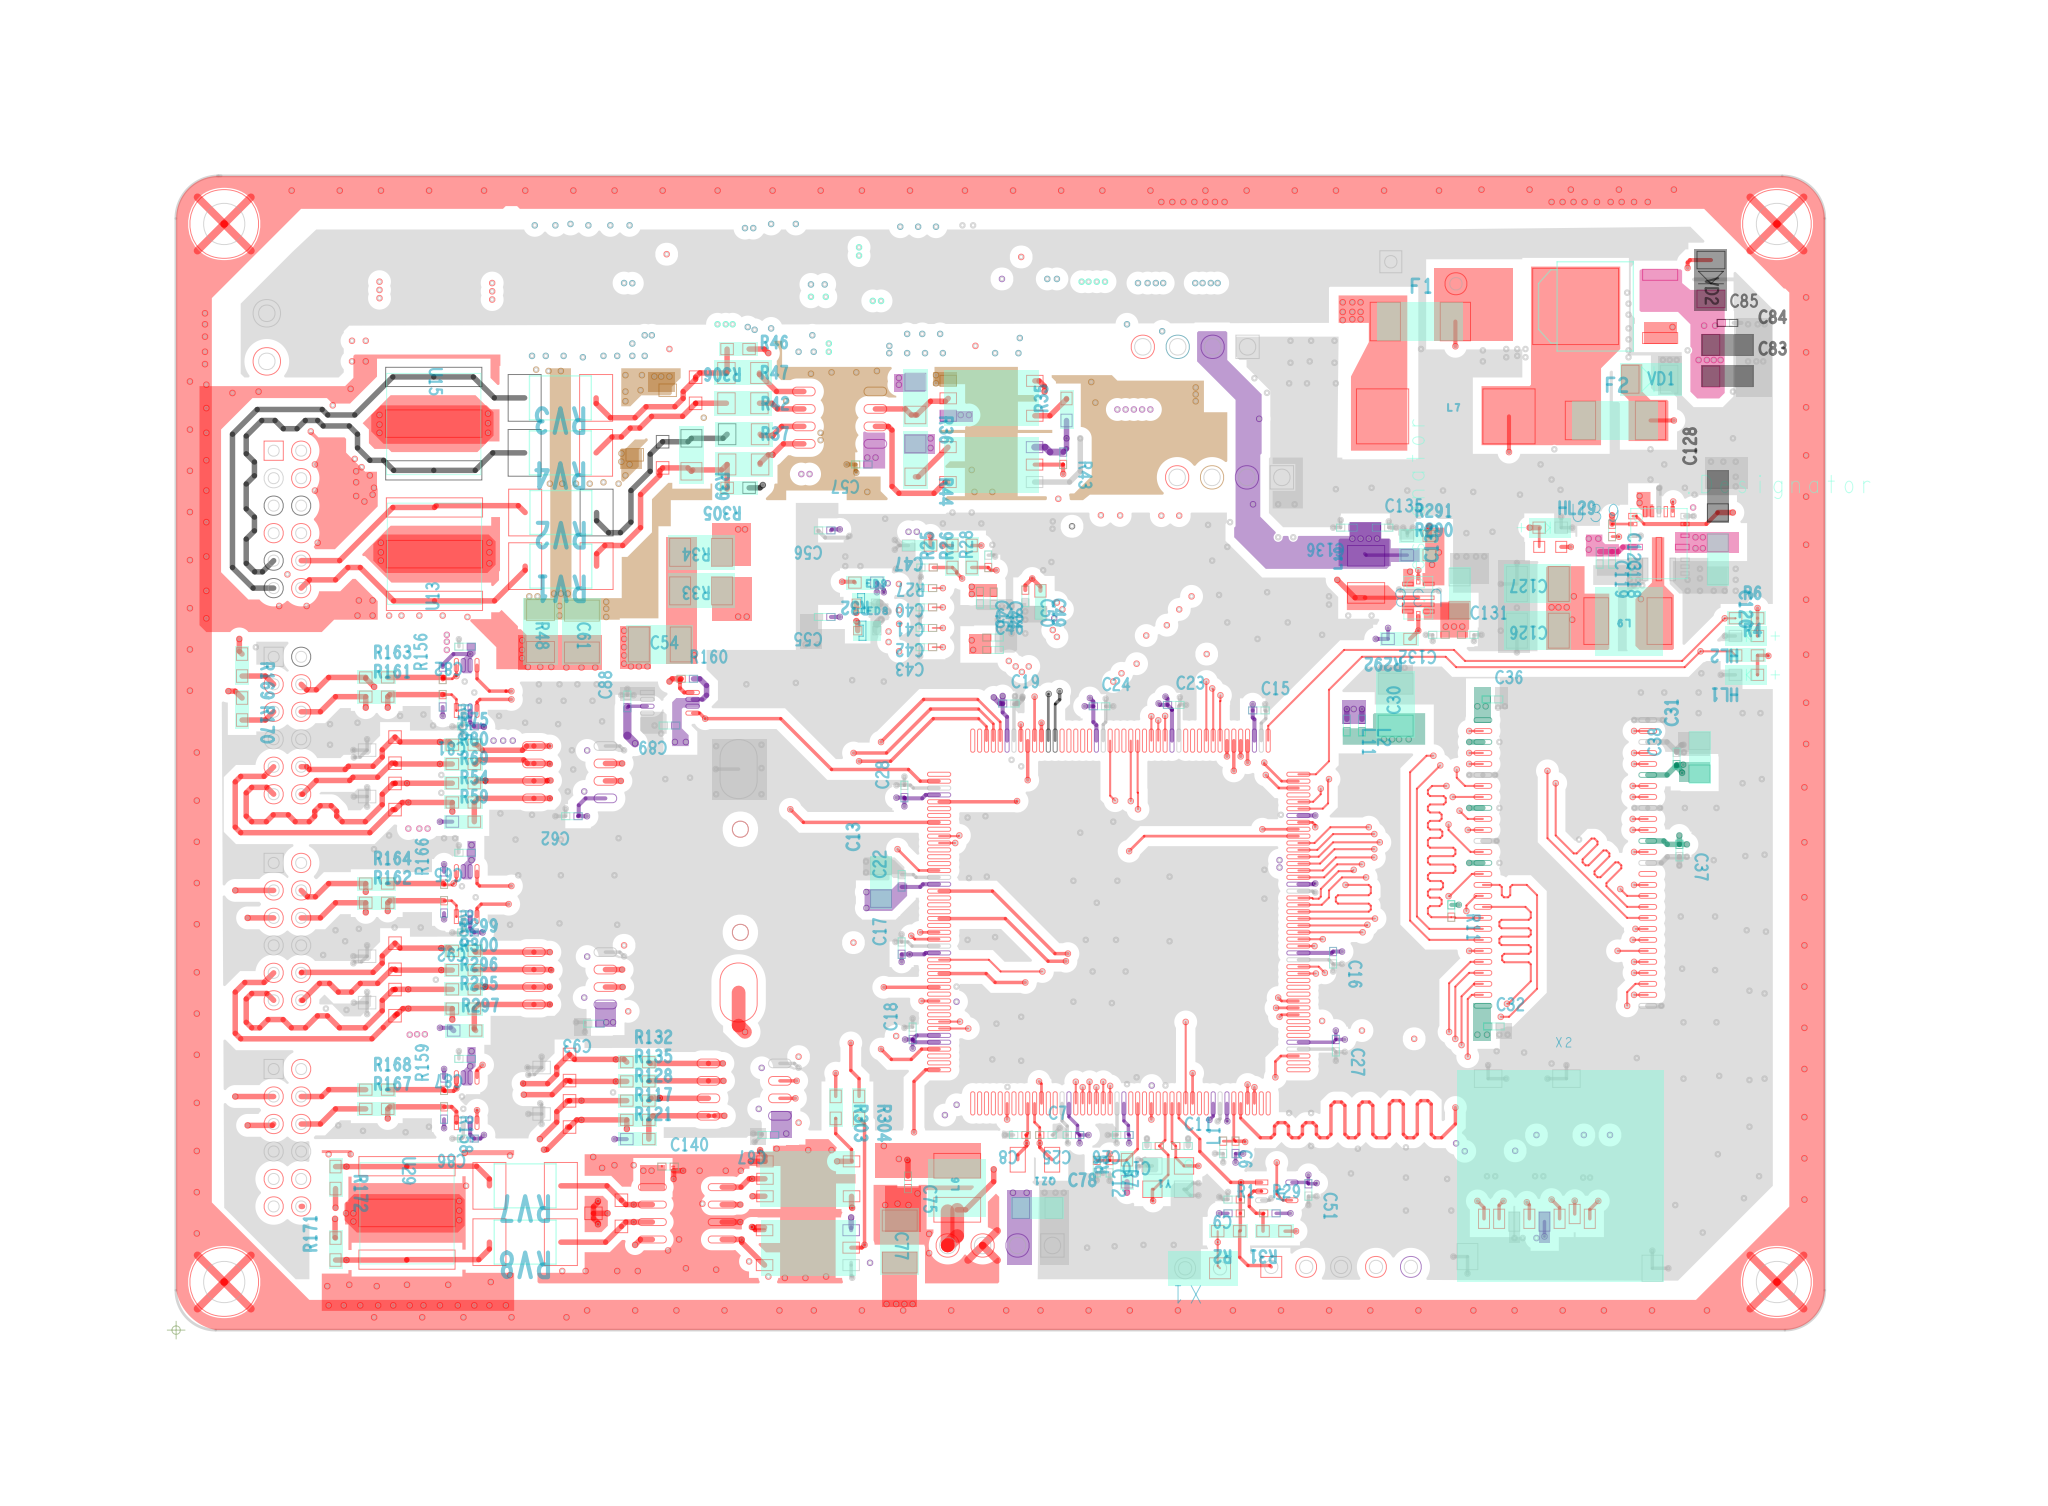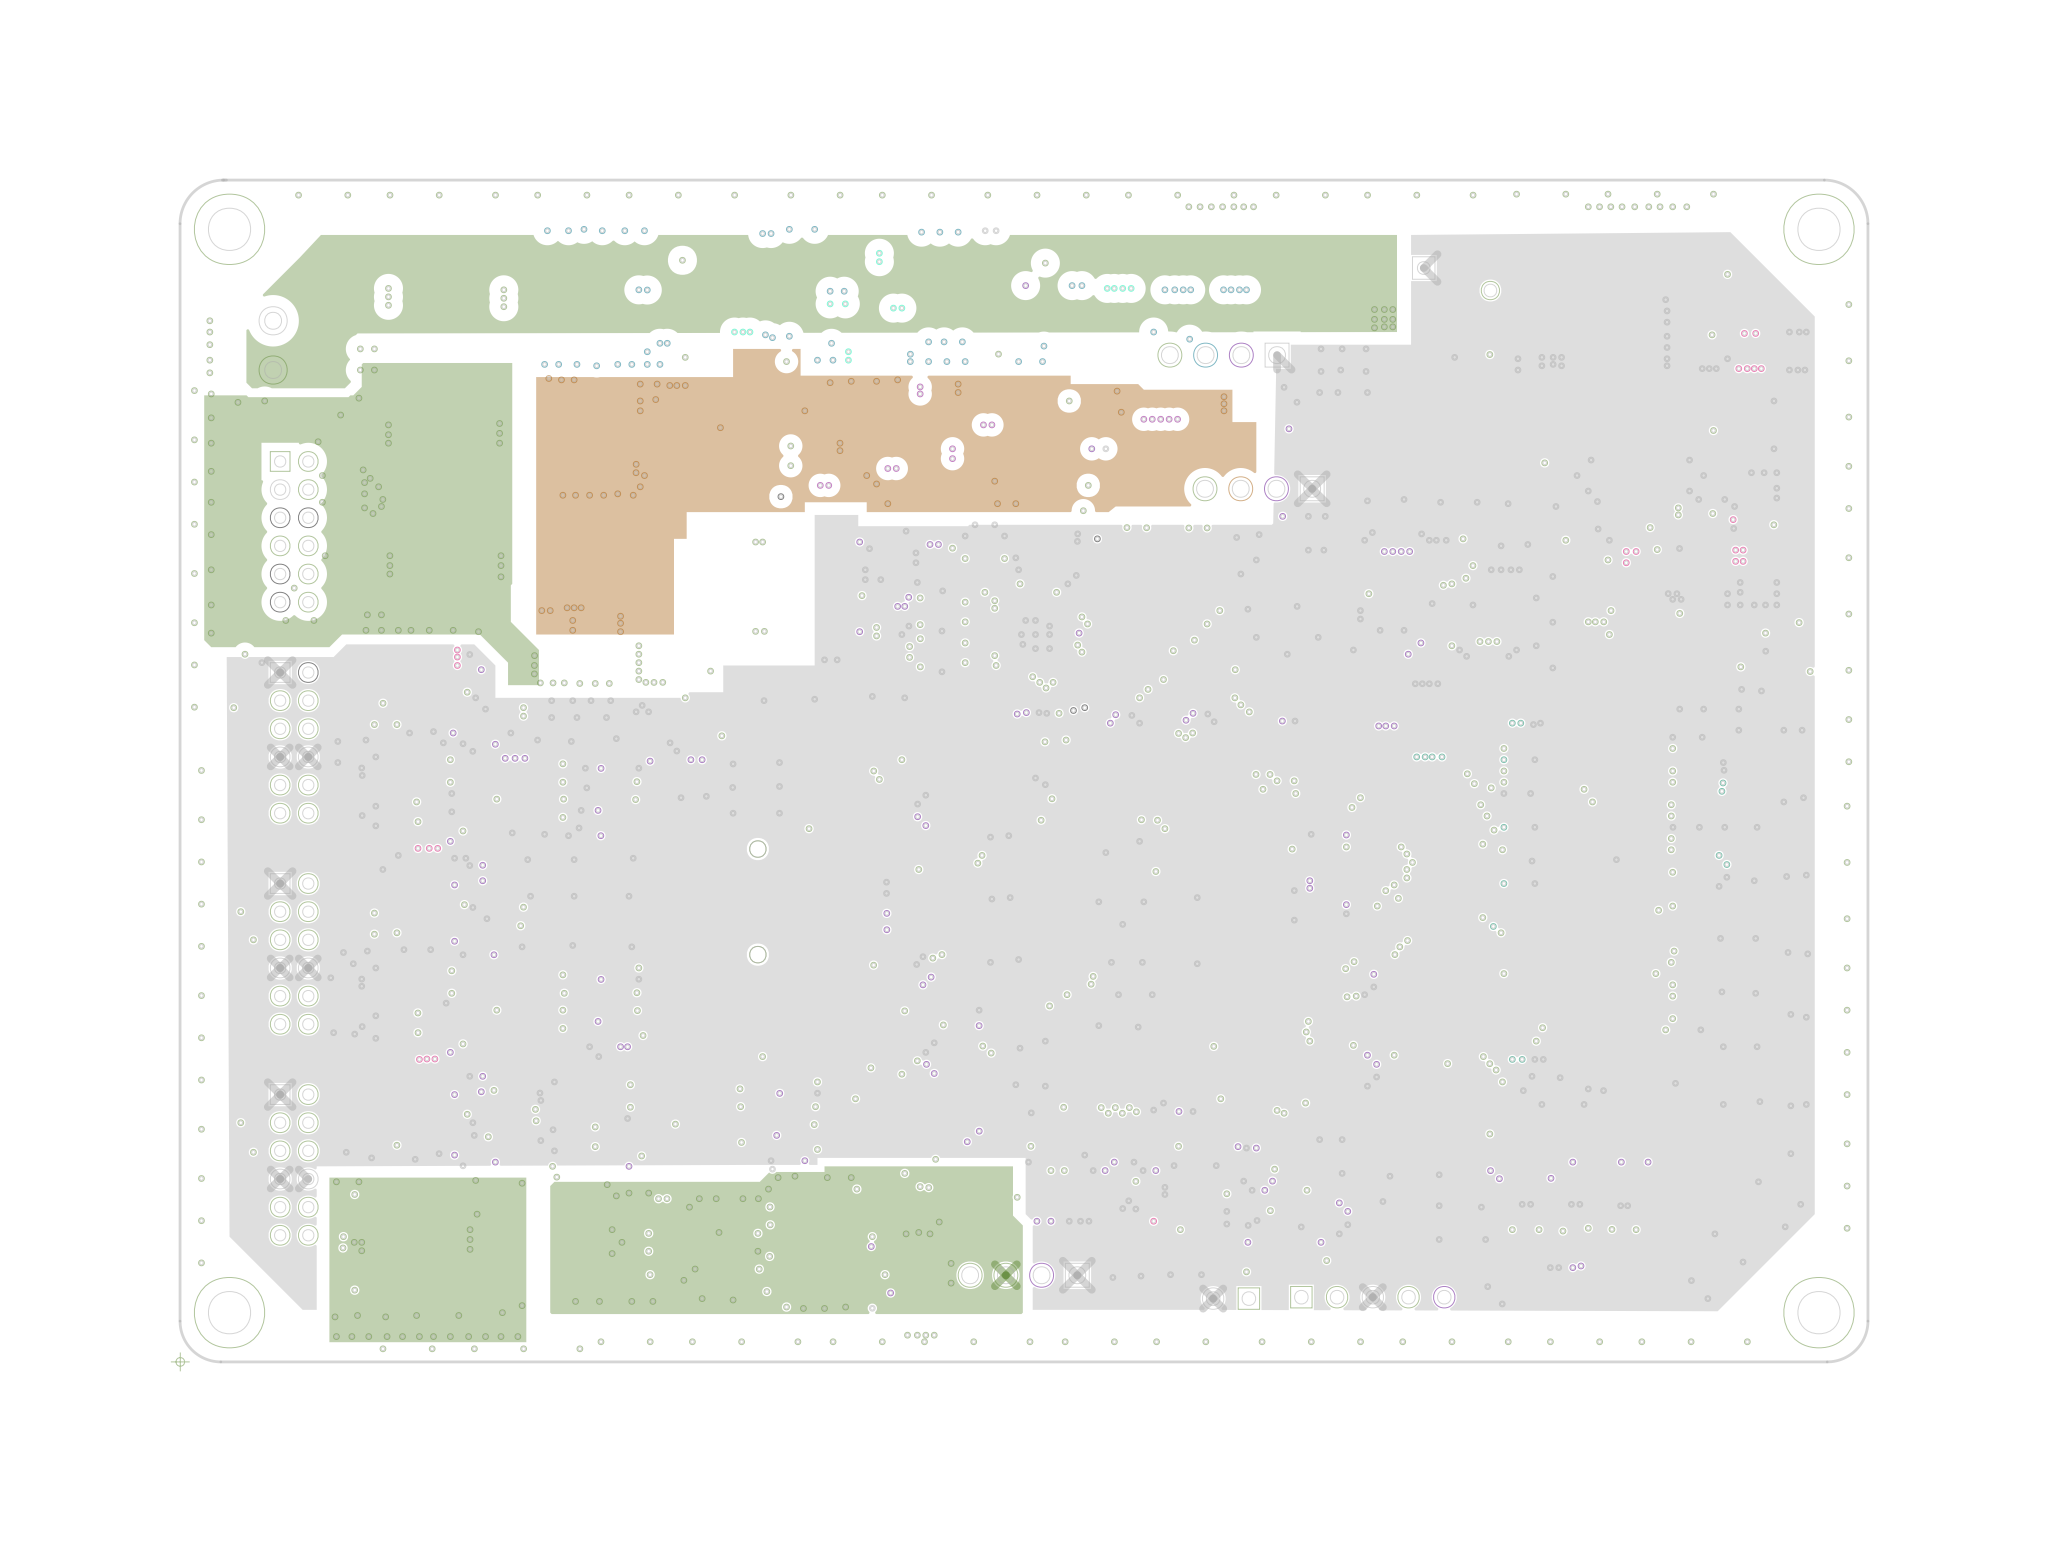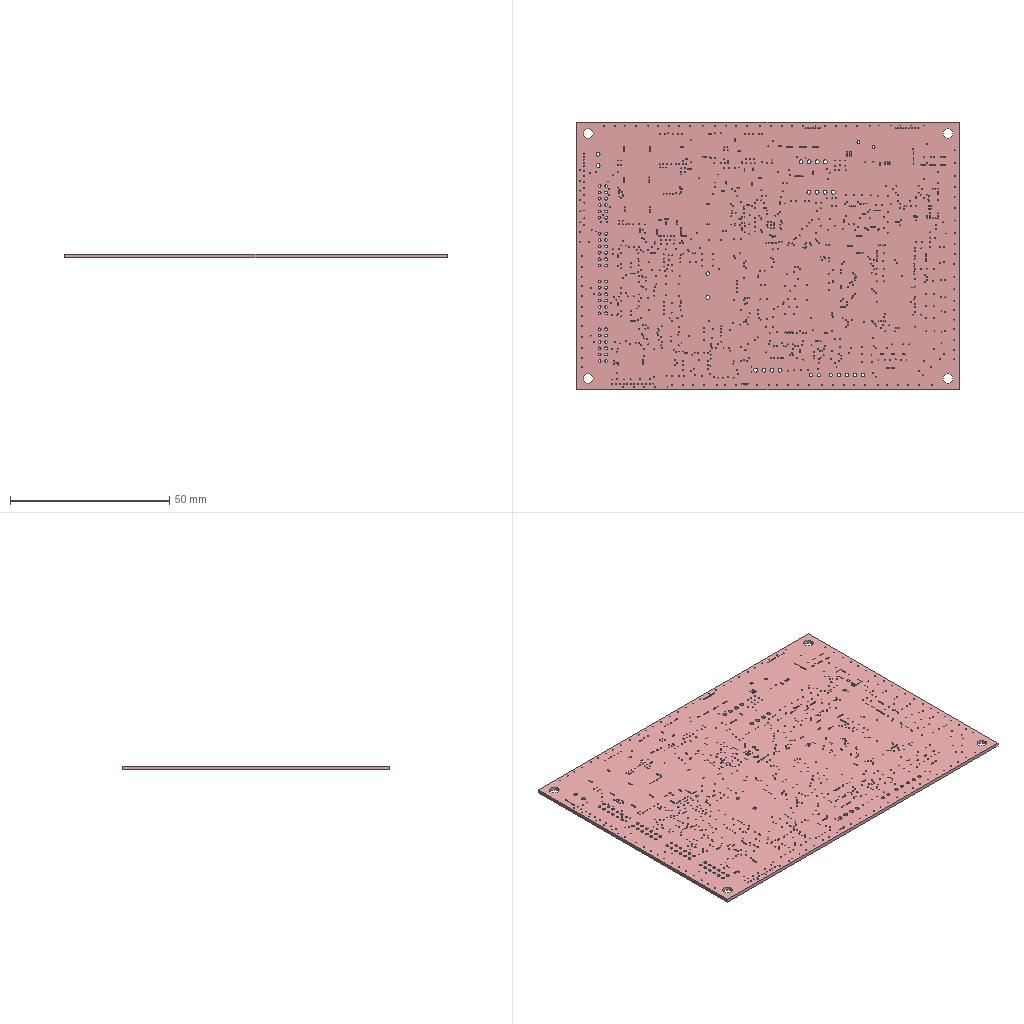Circuit board layout | Cadence Allegro | box 120.2 x 84.2 x 1.1 mm
Layer stack:
# Cadence Allegro layer stack of  (unit mm; from the constraint file cross-section; dielectric type: 0 not recorded (Allegro does not mark core vs prepreg), 3 surface material)
index,name,kind,layer,copper_thickness_mm,dielectric_type,dielectric_thickness_mm,dielectric_material,dielectric_constant
0,Top Surface,other,,,,,,
1,TOP,copper,TOP,0.0305,,,,
2,Dielectric1,dielectric,,,0,0.2032,FR-4,4.5
3,GND02,copper,GND02,0.0305,,,,
4,Dielectric2,dielectric,,,0,0.2032,FR-4,4.5
5,LAYER03,copper,LAYER03,0.0305,,,,
6,Dielectric3,dielectric,,,0,0.2032,FR-4,4.5
7,POWER04,copper,POWER04,0.0305,,,,
8,Dielectric4,dielectric,,,0,0.2032,FR-4,4.5
9,GND05,copper,GND05,0.0305,,,,
10,Dielectric5,dielectric,,,0,0.2032,FR-4,4.5
11,BOTTOM,copper,BOTTOM,0.0305,,,,
12,Bottom Surface,other,,,,,,
# drill layer pairs: low layer,high layer
drill_pair,TOP,BOTTOM
Part placement, first 474 of 522 lines:
REFDES,COMP_VALUE,SYM_NAME,SYM_X,SYM_Y,SYM_ROTATE,SYM_MIRROR
C1,2.2uf/16V,C0603,61.500,42.500,90.000,YES
C2,2.2uf/16V,C0603,81.200,36.700,0.000,YES
C3,1nf/50V,C0402,60.500,15.850,270.000,YES
C4,2.2uf/16V,C0603,76.200,14.400,0.000,YES
C5,0.1uf/50V,C0402,75.450,16.100,180.000,YES
C6,0.1uf/50V,C0402,76.200,13.750,270.000,NO
C7,6pf/50V,C0402,62.850,14.200,0.000,NO
C8,6pf/50V,C0402,61.850,14.200,180.000,NO
C9,0.1uf/50V,C0402,77.450,9.500,180.000,NO
C10,22pf/50V,C0402,71.550,13.400,180.000,NO
C11,22pf/50V,C0402,72.750,13.400,0.000,NO
C12,10nf/50V,C0402,67.000,12.350,270.000,NO
C13,4.7uf/50V,C0805,51.300,32.600,90.000,NO
C14,0.1uf/50V,C0402,83.600,32.650,90.000,YES
C15,0.1uf/50V,C0402,78.350,45.100,0.000,NO
C16,0.1uf/50V,C0402,84.200,27.550,270.000,NO
C17,0.1uf/50V,C0402,52.800,27.350,90.000,NO
C18,0.1uf/50V,C0402,53.600,21.150,90.000,NO
C19,0.1uf/50V,C0402,60.150,45.600,0.000,NO
C20,0.1uf/50V,C0402,82.150,37.900,0.000,YES
C21,4.7uf/50V,C0805,80.400,32.400,0.000,YES
C22,0.1uf/50V,C0402,52.800,32.250,90.000,NO
C23,0.1uf/50V,C0402,72.150,45.500,0.000,NO
C24,0.1uf/50V,C0402,66.750,45.400,0.000,NO
C25,0.1uf/50V,C0402,65.750,14.200,180.000,NO
C26,0.1uf/50V,C0402,69.350,14.200,180.000,NO
C27,0.1uf/50V,C0402,84.400,21.150,270.000,NO
C28,0.1uf/50V,C0402,53.000,38.750,90.000,NO
C29,10nf/50V,C0402,72.000,16.050,270.000,YES
C30,22uf/16V,C1210,88.751,45.512,90.000,NO
C31,4.7uf/50V,C0805,110.869,41.688,90.000,NO
C32,0.1uf/50V,C0402,95.450,22.100,0.000,NO
C33,0.1uf/50V,C0402,94.750,34.000,180.000,YES
C34,0.1uf/50V,C0402,94.750,38.000,180.000,YES
C35,0.1uf/50V,C0402,94.750,42.800,180.000,YES
C36,0.1uf/50V,C0402,95.350,45.900,0.000,NO
C37,0.1uf/50V,C0402,109.400,35.350,270.000,NO
C38,0.1uf/50V,C0402,109.200,41.150,90.000,NO
C39,0.1uf/50V,C0402,98.950,7.300,0.000,YES
C40,NC/10pF,C0402,55.050,54.000,180.000,NO
C41,NC/10pF,C0402,55.050,52.600,180.000,NO
C42,NC/10pF,C0402,55.050,51.100,180.000,NO
C43,NC/10pF,C0402,55.050,49.700,180.000,NO
C44,0.1uf/50V,C0402,59.500,53.700,270.000,NO
C45,0.1uf/50V,C0402,58.500,53.750,270.000,NO
C46,0.1uf/50V,C0402,59.000,49.500,0.000,NO
C47,10uf/16V,C0603,54.100,57.100,180.000,NO
C48,0.1uf/50V,C0402,59.000,50.400,0.000,NO
C49,10uf/16V,C0603,62.900,53.000,270.000,NO
C50,0.1uf/50V,C0402,61.800,53.850,270.000,NO
C51,0.1uf/50V,C0402,82.400,10.650,270.000,NO
C52,22pf/50V,C0402,61.050,55.900,0.000,YES
C53,22pf/50V,C0402,62.200,55.900,180.000,YES
C54,1NF/2KV,C1210,35.200,49.900,0.000,NO
C55,0.1uf/50V,C0402,47.650,51.900,180.000,NO
C56,0.1uf/50V,C0402,47.650,58.200,180.000,NO
C57,0.1uf/50V,C0402,50.350,63.000,180.000,NO
C58,4.7uf/50V,C0805,79.572,58.912,180.000,YES
C59,0.1uf/50V,C0402,67.799,66.962,0.000,YES
C60,10uf/16V,C0603,67.844,68.289,0.000,YES
C61,1NF/2KV,C1210,29.532,50.837,270.000,NO
C62,0.1uf/50V,C0402,29.250,37.400,180.000,NO
C65,0.1uf/50V,C0402,21.479,34.738,180.000,NO
C67,0.1uf/50V,C0402,43.550,14.200,180.000,NO
C69,0.1uf/50V,C0402,46.700,75.250,270.000,YES
C70,22pf/50V,C0402,35.200,71.350,270.000,YES
C71,1NF/2KV,C1210,72.400,78.900,270.000,YES
C72,4.7uf/50V,C0805,77.272,68.212,180.000,YES
C73,0.1uf/50V,C0402,68.550,76.700,180.000,YES
C74,10uf/16V,C0603,69.000,78.100,180.000,YES
C75,0.1uf/50V,C0402,53.262,11.199,270.000,NO
C76,22pf/50V,C0402,29.450,12.000,180.000,YES
C77,1NF/2KV,C1210,52.663,6.449,270.000,NO
C78,4.7uf/50V,C0805,62.672,8.888,0.000,NO
C79,0.1uf/50V,C0402,40.350,9.200,0.000,YES
C80,10uf/16V,C0603,53.211,10.744,90.000,YES
C81,0.1uf/50V,C0402,21.694,43.938,180.000,NO
C82,0.1uf/50V,C0402,21.479,49.738,180.000,NO
C83,10uf/50V,C0805,112.900,69.400,0.000,NO
C84,10uf/50V,C0805,112.900,71.700,0.000,NO
C85,0.1uf/50V,C0402,112.450,73.300,0.000,NO
C86,0.1uf/50V,C0402,21.694,13.938,180.000,NO
C87,0.1uf/50V,C0402,21.479,19.738,180.000,NO
C88,0.1uf/50V,C0402,32.838,45.306,90.000,NO
C89,0.1uf/50V,C0402,36.350,44.000,180.000,NO
C90,4.7uf/50V,C0805,19.500,46.100,180.000,YES
C91,4.7uf/50V,C0805,19.600,31.200,180.000,YES
C92,0.1uf/50V,C0402,21.694,28.938,180.000,NO
C93,0.1uf/50V,C0402,30.850,22.300,180.000,NO
C94,4.7uf/50V,C0805,18.500,16.400,180.000,YES
C115,10nf/50V,C0402,109.300,56.850,90.000,YES
C116,0.1uf/50V,C0402,110.200,56.850,90.000,YES
C117,0.1uf/50V,C0402,110.200,57.850,270.000,YES
C118,0.1uf/50V,C0402,104.500,56.650,270.000,NO
C119,10nf/50V,C0402,103.600,56.650,270.000,NO
C120,10uf/50V,C0805,112.200,56.100,270.000,NO
C121,10uf/50V,C0805,105.000,56.000,180.000,YES
C122,10uf/50V,C0805,112.200,56.100,90.000,YES
C123,0.47uf/25V,C0402,104.500,58.650,270.000,NO
C124,0.1uf/50V,C0402,107.050,60.700,180.000,YES
C125,22uf/16V,C1210,99.100,50.900,0.000,YES
C126,22uf/16V,C1210,99.100,50.900,180.000,NO
C127,22uf/16V,C1210,99.100,54.300,180.000,NO
C128,4.7uf/50V,C0805,112.200,60.700,90.000,NO
C129,0.1uf/50V,C0402,107.050,59.800,180.000,YES
C130,22uf/16V,C1210,94.100,53.700,270.000,YES
C131,10nf/50V,C0402,93.550,50.600,0.000,NO
C132,0.1uf/50V,C0402,92.350,50.600,180.000,NO
C133,10uf/50V,C0805,93.400,53.600,90.000,NO
C134,22pf/50V,C0402,91.150,56.400,0.000,YES
C135,0.1uf/50V,C0402,87.350,58.400,0.000,NO
C136,0.1uf/50V,C0402,85.650,58.400,180.000,NO
C137,22uf/16V,C1210,86.600,55.000,90.000,YES
C138,10nf/50V,C0402,90.300,54.550,90.000,YES
C139,0.1uf/50V,C0402,40.397,72.447,180.000,YES
C140,0.1uf/50V,C0402,35.350,11.900,0.000,NO
C141,1NF/2KV,C1210,110.300,77.600,270.000,YES
C142,10uf/50V,C0805,113.700,69.400,180.000,YES
C143,10uf/50V,C0805,113.700,71.700,180.000,YES
CN1,CR1220,CR1220,41.063,32.700,90.000,NO
D1,BAT54C,SOT23,57.686,16.600,270.000,YES
D2,SM712,SOT23,34.414,63.700,90.000,NO
D3,SM712,SOT23,36.814,68.400,90.000,NO
D5,SM712,SOT23,14.940,38.831,90.000,NO
D7,SM712,SOT23,14.940,42.210,90.000,NO
D14,SM712,SOT23,27.640,15.731,90.000,NO
D16,SM712,SOT23,27.640,19.110,90.000,NO
D18,SMC24,SOT23,33.914,75.400,90.000,YES
D19,TJA1044GT/3,SO8,44.940,77.605,0.000,YES
D20,SMC24,SOT23,31.414,8.500,90.000,NO
D21,TJA1044GT/3,SO8,39.740,6.595,180.000,NO
D22,TXS0102DCUR,VSSOP8,20.397,45.089,90.000,NO
D23,TXS0102DCUR,VSSOP8,20.397,15.089,90.000,NO
D24,TXS0102DCUR,VSSOP8,34.289,46.403,0.000,NO
D25,TXS0102DCUR,VSSOP8,20.397,30.089,90.000,NO
D26,SM712,SOT23,14.940,23.831,90.000,NO
D27,SM712,SOT23,14.940,27.210,90.000,NO
ED8,ESD9X5VU,ESD5Z12T1,49.600,50.900,0.000,NO
ED9,ESD9X5VU,ESD5Z12T1,49.500,52.900,0.000,NO
ED10,ESD9X5VU,ESD5Z12T1,49.200,57.000,90.000,YES
ED11,ESD9X5VU,ESD5Z12T1,49.300,59.500,270.000,YES
F1,JFC2410-2100TS,JFC2410-2100TS,88.000,73.400,0.000,NO
F2,JFC2410-2100TS,JFC2410-2100TS,102.200,66.200,0.000,NO
F3,SMD1812P150TF/33,1812_2,15.500,49.100,180.000,YES
F4,SMD1812P150TF/33,1812_2,15.200,34.500,180.000,YES
F5,SMD1812P150TF/33,1812_2,15.200,19.500,180.000,YES
HL1,LED,LED0603,114.279,47.688,180.000,NO
HL2,LED,LED0603,114.279,50.515,180.000,NO
HL3,LED,LED0603,56.500,57.900,270.000,YES
HL4,LED,LED0603,57.900,57.900,270.000,YES
HL29,LED,LED0603,100.000,58.400,0.000,NO
HOLE1,HOLE,HOLEPAD_50X30,116.500,3.500,0.000,NO
HOLE2,HOLE,HOLEPAD_50X30,116.500,80.500,0.000,NO
HOLE3,HOLE,HOLEPAD_50X30,3.500,3.500,0.000,NO
HOLE4,HOLE,HOLEPAD_50X30,3.500,80.500,0.000,NO
J1,SIP5_2_1,SIP5,79.700,4.600,0.000,NO
L1,GZ1005D121TF,0402,77.100,12.850,90.000,NO
L2,GZ1005D601TF,0402,86.300,44.450,270.000,NO
L3,BLM18SG331TN1D,0603,54.100,57.100,0.000,YES
L4,WPN4020H1R0MT/5.8A,SM_IND_4,68.355,63.657,270.000,YES
L5,WPN4020H1R0MT/5.8A,SM_IND_4,65.655,73.257,270.000,YES
L6,WPN4020H1R0MT/5.8A,SM_IND_4,56.845,10.357,90.000,NO
L7,APS10A40M220,SM_IND_10X10,92.400,66.500,0.000,NO
L9,SMMS0530-2R2M/6.5A,SM_IND_5L,105.650,51.600,180.000,NO
L10,DFE252012PD-R47M=P2,SM_IND_3L,86.600,53.650,90.000,NO
L11,GZ1005D601TF,0402,85.200,44.450,270.000,NO
Q1,IRFR9024NTRPBF,TO252-2,104.000,74.500,180.000,NO
QZ1,XDMCZLNDDF-32.768KHZ,XTAL_SMD_3215,63.750,12.400,180.000,NO
R1,4.7K/1%,0402,76.550,8.500,0.000,NO
R2,100R/1%,0603,76.600,7.200,180.000,NO
R3,NC,0402,55.950,23.900,0.000,YES
R4,1K/1%,0603,114.289,49.107,0.000,NO
R5,100K/1%,0603,69.200,11.600,90.000,NO
R6,1K/1%,0603,114.289,51.810,0.000,NO
R7,10K/1%,0402,67.933,12.342,270.000,NO
R8,10K/1%,0402,55.050,25.000,180.000,YES
R9,10K/1%,0402,71.000,16.950,90.000,YES
R10,SDNT1608X103F3450FTF,0603,69.900,16.800,270.000,YES
R11,10K/1%,0402,92.800,30.950,270.000,NO
R16,10K/1%,0402,93.781,13.592,180.000,YES
R17,10K/1%,0402,97.450,13.600,0.000,YES
R18,10K/1%,0402,99.150,13.600,180.000,YES
R19,10K/1%,0402,102.450,13.600,0.000,YES
R20,10K/1%,0402,104.350,13.600,0.000,YES
R21,49.9R/1%,0603,54.200,54.000,180.000,YES
R22,49.9R/1%,0603,54.200,52.600,180.000,YES
R23,49.9R/1%,0603,54.200,51.100,180.000,YES
R24,49.9R/1%,0603,54.200,49.700,180.000,YES
R25,1k,0603,56.500,56.300,90.000,NO
R26,1k,0603,57.900,56.300,90.000,NO
R27,4.7K/1%,0402,55.100,55.500,180.000,NO
R28,4.7K/1%,0402,59.100,55.500,90.000,NO
R29,4.7K/1%,0402,79.150,8.500,0.000,NO
R30,12.1K/1%,0603,54.200,55.400,0.000,YES
R31,0R,0603,79.900,7.200,180.000,NO
R32,NC,0603,50.200,54.400,180.000,NO
R33,75/5%,1206,38.200,53.800,180.000,NO
R34,75/5%,1206,38.200,56.600,180.000,NO
R35,220R,0603,64.800,67.000,90.000,NO
R36,1K/1%,0805,53.800,67.800,270.000,NO
R37,10R/1%,0805,41.300,63.000,0.000,NO
R38,825R/1%,0603,44.900,63.700,0.000,YES
R39,120R/1%,0805,37.500,63.700,270.000,NO
R40,825R/1%,0603,44.900,65.100,0.000,YES
R41,100R,0603,68.700,57.700,270.000,YES
R42,10R/1%,0805,41.300,65.200,0.000,NO
R43,10K/1%,0402,64.553,63.900,270.000,NO
R44,330R,0805,53.800,63.300,270.000,NO
R45,100R,0603,67.300,57.700,270.000,YES
R46,10R/1%,0805,41.248,69.655,0.000,NO
R47,10R/1%,0805,41.251,67.455,0.000,NO
R48,1M,1206,26.519,50.877,270.000,NO
R49,220R,0805,72.043,68.104,0.000,YES
R50,10K/1%,0402,30.400,39.050,270.000,YES
R51,10K/1%,0402,30.492,42.186,90.000,YES
R54,10R/1%,0603,20.900,38.400,0.000,NO
R59,825R/1%,0603,20.900,37.000,0.000,NO
R61,825R/1%,0603,20.900,39.800,180.000,YES
R62,100R/1%,0805,15.700,39.100,90.000,YES
R68,0R,0603,31.700,39.000,270.000,YES
R69,10R/1%,0603,20.900,39.800,0.000,NO
R74,0R,0603,31.700,42.200,90.000,YES
R75,10R/1%,0603,20.900,42.600,0.000,NO
R80,10R/1%,0603,20.900,41.200,0.000,NO
R83,10K/1%,0402,30.400,24.050,270.000,YES
R84,10K/1%,0402,30.492,27.186,90.000,YES
R87,NC,0603,70.100,57.700,270.000,YES
R90,NC,0603,65.900,57.700,270.000,YES
R94,NC,0603,20.900,37.000,0.000,YES
R95,NC,0603,20.900,42.600,0.000,YES
R96,NC,0603,21.000,21.800,0.000,YES
R97,NC,0603,20.900,27.600,0.000,YES
R98,0R,0603,31.700,24.000,270.000,YES
R101,NC,0603,33.600,13.900,0.000,YES
R102,NC,0603,33.600,19.500,0.000,YES
R103,0R,0603,31.700,27.200,90.000,YES
R115,10K/1%,0402,43.100,15.950,270.000,YES
R116,10K/1%,0402,43.192,19.086,90.000,YES
R117,10R/1%,0603,33.600,15.300,0.000,NO
R121,825R/1%,0603,33.600,13.900,0.000,NO
R122,100R/1%,0805,28.400,16.000,90.000,YES
R125,825R/1%,0603,33.600,16.700,180.000,YES
R127,0R,0603,44.400,15.900,270.000,YES
R128,10R/1%,0603,33.600,16.700,0.000,NO
R131,0R,0603,44.400,19.100,90.000,YES
R132,10R/1%,0603,33.600,19.500,0.000,NO
R135,10R/1%,0603,33.600,18.100,0.000,NO
R137,220R,0603,60.100,74.100,0.000,YES
R138,1K/1%,0805,48.700,72.700,270.000,YES
R139,1K/1%,0603,40.600,79.100,0.000,YES
R140,1K/1%,0603,59.400,77.300,270.000,YES
R141,499R,0805,48.700,77.300,90.000,YES
R142,62R/1%,1206,37.200,72.900,270.000,YES
R143,62R/1%,1206,37.200,78.200,90.000,YES
R144,1M,1206,75.300,78.900,270.000,YES
R145,220R,0805,65.000,77.500,180.000,YES
R146,220R,0603,49.200,10.500,90.000,YES
R147,1K/1%,0805,43.000,10.600,270.000,YES
R148,1K/1%,0603,35.000,6.600,0.000,YES
R149,1K/1%,0603,49.100,5.400,270.000,YES
R150,499R,0805,43.100,6.300,270.000,YES
R151,62R/1%,1206,30.700,10.100,180.000,YES
R152,62R/1%,1206,30.700,6.900,180.000,YES
R153,1M,1206,52.623,6.464,90.000,YES
R154,220R,0805,51.504,11.257,270.000,YES
R155,10K/1%,0402,19.400,46.250,270.000,NO
R156,10K/1%,0402,19.400,47.350,90.000,NO
R158,10K/1%,0402,19.500,16.250,270.000,NO
R159,10K/1%,0402,19.500,17.450,90.000,NO
R160,10K/1%,0402,36.750,47.400,0.000,NO
R161,100R/1%,0603,14.600,46.100,0.000,NO
R162,100R/1%,0603,14.600,31.100,0.000,NO
R163,100R/1%,0603,14.600,47.500,0.000,NO
R164,100R/1%,0603,14.600,32.500,0.000,NO
R165,10K/1%,0402,19.500,31.250,270.000,NO
R166,10K/1%,0402,19.500,32.450,90.000,NO
R167,100R/1%,0603,14.600,16.100,0.000,NO
R168,100R/1%,0603,14.600,17.500,0.000,NO
R169,NC,0603,4.800,48.400,270.000,NO
R170,NC,0603,4.800,45.200,270.000,NO
R171,0R,0603,11.600,5.900,90.000,NO
R172,0R,0603,11.600,11.100,270.000,NO
R287,10K/1%,0402,109.850,59.800,0.000,YES
R288,4.7K/1%,0402,109.850,60.700,0.000,YES
R289,1K/1%,R0603,100.000,57.000,180.000,NO
R290,88.7K/1%,0603,90.400,56.400,0.000,NO
R291,19.6K/1%,0603,90.400,57.800,0.000,NO
R292,10K/1%,0603,89.000,50.300,180.000,NO
R293,8.06K/1%,0402,89.500,53.650,270.000,YES
R294,100R/1%,0805,15.800,24.100,90.000,YES
R295,10R/1%,0603,20.900,23.400,0.000,NO
R296,10R/1%,0603,20.900,24.800,0.000,NO
R297,825R/1%,0603,21.000,21.800,0.000,NO
R298,825R/1%,0603,20.900,24.800,180.000,YES
R299,10R/1%,0603,20.900,27.600,0.000,NO
R300,10R/1%,0603,20.900,26.200,0.000,NO
R301,100R,0603,71.703,57.685,270.000,YES
R302,100R,0603,73.303,57.688,270.000,YES
R303,100R,0603,48.003,16.209,270.000,NO
R304,100R,0603,49.703,16.206,270.000,NO
R305,NC,0603,40.900,61.297,180.000,NO
R306,NC,0603,40.897,71.397,180.000,NO
R307,1M,1206,107.000,77.600,270.000,YES
R309,10K/1%,0603,109.700,73.900,180.000,YES
R310,47K/1%,0603,109.700,72.200,0.000,YES
RV1,SMD1812P050TF,1812_2,28.000,55.600,180.000,NO
RV2,SMD1812P050TF,1812_2,28.000,59.500,180.000,NO
RV3,SMD1812P050TF,1812_2,27.965,67.843,180.000,NO
RV4,SMD1812P050TF,1812_2,27.962,63.843,180.000,NO
RV5,SMD1812P050TF,1812_2,27.900,73.400,0.000,YES
RV6,SMD1812P050TF,1812_2,27.900,77.400,0.000,YES
RV7,SMD1812P050TF,1812_2,25.400,10.500,180.000,NO
RV8,SMD1812P050TF,1812_2,25.400,6.400,180.000,NO
RV9,820KD07J,10D151K,88.400,77.750,180.000,YES
T1,HX1188NL,TRANS_H1102,46.583,59.545,0.000,YES
TP1,TESTPOINT,TESTPOINT-33MIL,86.600,60.300,0.000,YES
TP2,TESTPOINT,TESTPOINT-33MIL,110.000,49.400,0.000,YES
TP3,TESTPOINT,TESTPOINT-33MIL,113.600,51.800,0.000,YES
TP4,TESTPOINT,TESTPOINT-33MIL,116.300,49.600,0.000,YES
TP5,TESTPOINT,TESTPOINT-33MIL,116.300,52.400,0.000,YES
TP6,TESTPOINT,TESTPOINT-33MIL,84.800,7.100,0.000,YES
TP7,TESTPOINT,TESTPOINT-33MIL,68.900,12.300,0.000,YES
TP8,TESTPOINT,TESTPOINT-33MIL,53.700,25.000,0.000,YES
TP9,TESTPOINT,TESTPOINT-33MIL,72.000,14.600,0.000,YES
TP10,TESTPOINT,TESTPOINT-33MIL,87.300,8.200,0.000,YES
TP11,TESTPOINT,TESTPOINT-33MIL,82.800,7.200,0.000,YES
TP13,TESTPOINT,TESTPOINT-33MIL,76.700,6.400,0.000,YES
TP14,TESTPOINT,TESTPOINT-33MIL,78.300,10.800,0.000,YES
TP15,TESTPOINT,TESTPOINT-33MIL,56.700,19.300,0.000,YES
TP17,TESTPOINT,TESTPOINT-33MIL,59.800,43.300,0.000,YES
TP18,TESTPOINT,TESTPOINT-33MIL,62.000,15.800,0.000,YES
TP19,TESTPOINT,TESTPOINT-33MIL,78.500,13.700,0.000,YES
TP20,TESTPOINT,TESTPOINT-33MIL,81.600,29.900,0.000,YES
TP21,TESTPOINT,TESTPOINT-33MIL,70.300,9.500,0.000,YES
TP22,TESTPOINT,TESTPOINT-33MIL,73.500,12.000,0.000,YES
TP23,TESTPOINT,TESTPOINT-33MIL,61.500,12.800,0.000,YES
TP24,TESTPOINT,TESTPOINT-33MIL,63.300,12.800,0.000,YES
TP25,TESTPOINT,TESTPOINT-33MIL,103.700,8.500,0.000,YES
TP26,TESTPOINT,TESTPOINT-33MIL,101.900,8.500,0.000,YES
TP27,TESTPOINT,TESTPOINT-33MIL,100.100,8.500,0.000,YES
TP28,TESTPOINT,TESTPOINT-33MIL,98.300,8.600,0.000,YES
TP29,TESTPOINT,TESTPOINT-33MIL,96.500,8.600,0.000,YES
TP30,TESTPOINT,TESTPOINT-33MIL,94.700,8.600,0.000,YES
TP31,TESTPOINT,TESTPOINT-33MIL,50.500,57.600,0.000,YES
TP32,TESTPOINT,TESTPOINT-33MIL,50.500,58.900,0.000,YES
TP33,TESTPOINT,TESTPOINT-33MIL,49.500,50.700,0.000,YES
TP34,TESTPOINT,TESTPOINT-33MIL,49.500,53.200,0.000,YES
TP37,TESTPOINT,TESTPOINT-33MIL,53.300,48.000,0.000,YES
TP38,TESTPOINT,TESTPOINT-33MIL,53.300,59.400,0.000,YES
TP39,TESTPOINT,TESTPOINT-33MIL,55.100,59.400,0.000,YES
TP40,TESTPOINT,TESTPOINT-33MIL,56.900,55.600,0.000,YES
TP41,TESTPOINT,TESTPOINT-33MIL,58.700,55.600,0.000,YES
TP42,TESTPOINT,TESTPOINT-33MIL,80.700,7.100,0.000,YES
TP43,TESTPOINT,TESTPOINT-33MIL,75.000,48.200,0.000,YES
TP44,TESTPOINT,TESTPOINT-33MIL,57.800,46.100,0.000,YES
TP45,TESTPOINT,TESTPOINT-33MIL,57.600,47.900,0.000,YES
TP46,TESTPOINT,TESTPOINT-33MIL,73.900,51.500,0.000,YES
TP47,TESTPOINT,TESTPOINT-33MIL,73.000,49.900,0.000,YES
TP48,TESTPOINT,TESTPOINT-33MIL,72.100,48.300,0.000,YES
TP49,TESTPOINT,TESTPOINT-33MIL,68.800,46.100,0.000,YES
TP50,TESTPOINT,TESTPOINT-33MIL,69.900,47.600,0.000,YES
TP51,TESTPOINT,TESTPOINT-33MIL,70.600,49.800,0.000,YES
TP52,TESTPOINT,TESTPOINT-33MIL,61.100,47.100,0.000,YES
TP53,TESTPOINT,TESTPOINT-33MIL,60.500,60.300,0.000,YES
TP54,TESTPOINT,TESTPOINT-33MIL,64.400,57.100,0.000,YES
TP55,TESTPOINT,TESTPOINT-33MIL,51.600,56.000,0.000,YES
TP56,TESTPOINT,TESTPOINT-33MIL,49.500,54.500,0.000,YES
TP66,TESTPOINT,TESTPOINT-33MIL,36.400,49.100,0.000,YES
TP93,TESTPOINT,TESTPOINT-33MIL,33.400,39.700,0.000,YES
TP94,TESTPOINT,TESTPOINT-33MIL,33.400,41.500,0.000,YES
TP95,TESTPOINT,TESTPOINT-33MIL,17.600,38.400,0.000,YES
TP96,TESTPOINT,TESTPOINT-33MIL,26.400,38.700,0.000,YES
TP97,TESTPOINT,TESTPOINT-33MIL,28.000,40.000,0.000,YES
TP98,TESTPOINT,TESTPOINT-33MIL,17.600,40.200,0.000,YES
TP99,TESTPOINT,TESTPOINT-33MIL,18.500,42.800,0.000,YES
TP100,TESTPOINT,TESTPOINT-33MIL,20.000,41.200,0.000,YES
TP101,TESTPOINT,TESTPOINT-33MIL,27.900,42.500,0.000,YES
TP102,TESTPOINT,TESTPOINT-33MIL,26.300,41.200,0.000,YES
TP103,TESTPOINT,TESTPOINT-33MIL,33.200,24.900,0.000,YES
TP104,TESTPOINT,TESTPOINT-33MIL,29.200,26.300,0.000,YES
TP105,TESTPOINT,TESTPOINT-33MIL,23.300,22.300,0.000,YES
TP106,TESTPOINT,TESTPOINT-33MIL,23.300,27.600,0.000,YES
TP107,TESTPOINT,TESTPOINT-33MIL,17.600,23.100,0.000,YES
TP108,TESTPOINT,TESTPOINT-33MIL,17.600,25.000,0.000,YES
TP109,TESTPOINT,TESTPOINT-33MIL,18.600,27.900,0.000,YES
TP110,TESTPOINT,TESTPOINT-33MIL,18.600,26.200,0.000,YES
TP111,TESTPOINT,TESTPOINT-33MIL,27.900,27.500,0.000,YES
TP112,TESTPOINT,TESTPOINT-33MIL,26.500,26.200,0.000,YES
TP113,TESTPOINT,TESTPOINT-33MIL,26.400,23.700,0.000,YES
TP114,TESTPOINT,TESTPOINT-33MIL,28.000,25.000,0.000,YES
TP115,TESTPOINT,TESTPOINT-33MIL,41.800,16.700,0.000,YES
TP116,TESTPOINT,TESTPOINT-33MIL,41.800,18.500,0.000,YES
TP117,TESTPOINT,TESTPOINT-33MIL,36.000,13.900,0.000,YES
TP118,TESTPOINT,TESTPOINT-33MIL,35.900,19.500,0.000,YES
TP119,TESTPOINT,TESTPOINT-33MIL,40.600,15.600,0.000,YES
TP120,TESTPOINT,TESTPOINT-33MIL,36.000,16.900,0.000,YES
TP121,TESTPOINT,TESTPOINT-33MIL,30.200,15.100,0.000,YES
TP122,TESTPOINT,TESTPOINT-33MIL,30.200,16.800,0.000,YES
TP123,TESTPOINT,TESTPOINT-33MIL,40.400,19.600,0.000,YES
TP124,TESTPOINT,TESTPOINT-33MIL,40.200,17.600,0.000,YES
TP125,TESTPOINT,TESTPOINT-33MIL,31.300,18.100,0.000,YES
TP126,TESTPOINT,TESTPOINT-33MIL,31.300,19.900,0.000,YES
TP127,TESTPOINT,TESTPOINT-33MIL,60.100,72.700,0.000,YES
TP128,TESTPOINT,TESTPOINT-33MIL,58.800,71.600,0.000,YES
TP129,TESTPOINT,TESTPOINT-33MIL,56.000,22.600,0.000,YES
TP130,TESTPOINT,TESTPOINT-33MIL,60.800,78.100,0.000,YES
TP131,TESTPOINT,TESTPOINT-33MIL,62.600,71.600,0.000,YES
TP132,TESTPOINT,TESTPOINT-33MIL,66.200,79.500,0.000,YES
TP133,TESTPOINT,TESTPOINT-33MIL,39.800,80.600,0.000,YES
TP134,TESTPOINT,TESTPOINT-33MIL,46.900,73.800,0.000,YES
TP135,TESTPOINT,TESTPOINT-33MIL,46.900,79.000,0.000,YES
TP136,TESTPOINT,TESTPOINT-33MIL,14.000,73.400,0.000,YES
TP137,TESTPOINT,TESTPOINT-33MIL,14.000,78.000,0.000,YES
TP138,TESTPOINT,TESTPOINT-33MIL,33.200,73.100,0.000,YES
TP139,TESTPOINT,TESTPOINT-33MIL,33.300,77.700,0.000,YES
TP140,TESTPOINT,TESTPOINT-33MIL,34.900,79.900,0.000,YES
TP141,TESTPOINT,TESTPOINT-33MIL,44.600,79.500,0.000,YES
TP142,TESTPOINT,TESTPOINT-33MIL,47.700,8.900,0.000,YES
TP143,TESTPOINT,TESTPOINT-33MIL,47.400,12.300,0.000,YES
TP144,TESTPOINT,TESTPOINT-33MIL,47.200,18.700,0.000,YES
TP145,TESTPOINT,TESTPOINT-33MIL,47.600,6.200,0.000,YES
TP146,TESTPOINT,TESTPOINT-33MIL,49.100,21.800,0.000,YES
TP147,TESTPOINT,TESTPOINT-33MIL,45.000,5.100,0.000,YES
TP148,TESTPOINT,TESTPOINT-33MIL,59.500,12.700,0.000,YES
TP149,TESTPOINT,TESTPOINT-33MIL,45.000,7.500,0.000,YES
TP150,TESTPOINT,TESTPOINT-33MIL,40.300,6.600,0.000,YES
TP151,TESTPOINT,TESTPOINT-33MIL,44.800,11.800,0.000,YES
TP152,TESTPOINT,TESTPOINT-33MIL,34.200,5.200,0.000,YES
TP153,TESTPOINT,TESTPOINT-33MIL,34.100,8.000,0.000,YES
TP154,TESTPOINT,TESTPOINT-33MIL,34.100,9.700,0.000,YES
TP155,TESTPOINT,TESTPOINT-33MIL,13.000,11.900,0.000,YES
TP156,TESTPOINT,TESTPOINT-33MIL,13.100,5.100,0.000,YES
TP157,TESTPOINT,TESTPOINT-33MIL,27.400,6.900,0.000,YES
TP158,TESTPOINT,TESTPOINT-33MIL,84.700,76.700,0.000,YES
TP159,TESTPOINT,TESTPOINT-33MIL,48.000,47.300,0.000,YES
TP160,TESTPOINT,TESTPOINT-33MIL,93.100,70.800,0.000,YES
TP161,TESTPOINT,TESTPOINT-33MIL,109.800,66.200,0.000,YES
TP162,TESTPOINT,TESTPOINT-33MIL,92.200,6.900,0.000,YES
TP163,TESTPOINT,TESTPOINT-33MIL,97.000,63.000,0.000,YES
TP164,TESTPOINT,TESTPOINT-33MIL,14.700,44.600,0.000,YES
TP165,TESTPOINT,TESTPOINT-33MIL,15.000,46.500,0.000,YES
TP166,TESTPOINT,TESTPOINT-33MIL,14.400,29.600,0.000,YES
TP167,TESTPOINT,TESTPOINT-33MIL,14.400,31.300,0.000,YES
TP168,TESTPOINT,TESTPOINT-33MIL,12.600,31.100,0.000,YES
TP169,TESTPOINT,TESTPOINT-33MIL,12.900,45.800,0.000,YES
TP170,TESTPOINT,TESTPOINT-33MIL,12.600,22.500,0.000,YES
TP171,TESTPOINT,TESTPOINT-33MIL,24.400,47.200,0.000,YES
TP172,TESTPOINT,TESTPOINT-33MIL,24.400,45.100,0.000,YES
TP173,TESTPOINT,TESTPOINT-33MIL,23.000,19.300,0.000,YES
TP174,TESTPOINT,TESTPOINT-33MIL,22.200,16.700,0.000,YES
TP175,TESTPOINT,TESTPOINT-33MIL,39.200,44.500,0.000,YES
TP176,TESTPOINT,TESTPOINT-33MIL,36.700,47.200,0.000,YES
TP177,TESTPOINT,TESTPOINT-33MIL,15.400,14.700,0.000,YES
TP178,TESTPOINT,TESTPOINT-33MIL,20.500,18.400,0.000,YES
TP179,TESTPOINT,TESTPOINT-33MIL,20.600,48.400,0.000,YES
TP180,TESTPOINT,TESTPOINT-33MIL,16.300,45.500,0.000,YES
TP181,TESTPOINT,TESTPOINT-33MIL,20.400,33.300,0.000,YES
TP182,TESTPOINT,TESTPOINT-33MIL,16.100,30.500,0.000,YES
TP183,TESTPOINT,TESTPOINT-33MIL,113.900,59.500,0.000,YES
TP184,TESTPOINT,TESTPOINT-33MIL,108.900,62.000,0.000,YES
TP186,TESTPOINT,TESTPOINT-33MIL,104.300,58.200,0.000,YES
TP187,TESTPOINT,TESTPOINT-33MIL,104.500,60.000,0.000,YES
TP188,TESTPOINT,TESTPOINT-33MIL,100.400,54.200,0.000,YES
TP189,TESTPOINT,TESTPOINT-33MIL,97.500,58.400,0.000,YES
TP190,TESTPOINT,TESTPOINT-33MIL,81.600,34.300,0.000,YES
TP191,TESTPOINT,TESTPOINT-33MIL,89.800,50.300,0.000,YES
TP192,TESTPOINT,TESTPOINT-33MIL,91.200,59.400,0.000,YES
TP193,TESTPOINT,TESTPOINT-33MIL,83.800,54.700,0.000,YES
TP194,TESTPOINT,TESTPOINT-33MIL,89.100,52.300,0.000,YES
TP195,TESTPOINT,TESTPOINT-33MIL,91.700,54.600,0.000,YES
TP196,TESTPOINT,TESTPOINT-33MIL,109.700,39.600,0.000,YES
TP197,TESTPOINT,TESTPOINT-33MIL,47.400,63.600,0.000,YES
TP198,TESTPOINT,TESTPOINT-33MIL,65.300,68.400,0.000,YES
Pad and via stacks:
# Allegro (Cadence) via spans and padstacks; design units: ("millimeters" 3 1000)
# via spans: padstack,start_layer,end_layer,net_example,count
VIA10X16MIL,ETCH/TOP,ETCH/BOTTOM,GND-E,1322
# Allegro padstack definitions: name,start_layer,end_layer,drill,plating,holeType,type
SR36X32,"ETCH/TOP","ETCH/TOP",0.0,"PLATED","none","smd"
SR2500X2400M,"ETCH/TOP","ETCH/TOP",0.0,"PLATED","none","smd"
SR36X36,"ETCH/TOP","ETCH/TOP",0.0,"PLATED","none","smd"
SR1000X800M,"ETCH/TOP","ETCH/TOP",0.0,"PLATED","none","smd"
SR1500X600M,"ETCH/TOP","ETCH/TOP",0.0,"PLATED","none","smd"
SR2700X1500M,"ETCH/TOP","ETCH/TOP",0.0,"PLATED","none","smd"
SR60X100,"ETCH/TOP","ETCH/TOP",0.0,"PLATED","none","smd"
CO60X35,"ETCH/TOP","ETCH/BOTTOM",3.5,"PLATED","circle_drill","through"
TS1000X600M,"ETCH/TOP","ETCH/BOTTOM",0.6,"PLATED","circle_drill","through"
TC1000X600M,"ETCH/TOP","ETCH/BOTTOM",0.6,"PLATED","circle_drill","through"
CO50X30,"ETCH/TOP","ETCH/BOTTOM",3.0,"PLATED","circle_drill","through"
VIA22D12,"ETCH/TOP","ETCH/BOTTOM",0.305,"PLATED","circle_drill","through"
VIA20D10,"ETCH/TOP","ETCH/BOTTOM",0.254,"PLATED","circle_drill","through"
SMDS0R8X0R8MM,"ETCH/TOP","ETCH/TOP",0.0,"NON_PLATED","none","smd"
SMD0R46X0R5MM,"ETCH/TOP","ETCH/TOP",0.0,"NON_PLATED","none","smd"
SR60X50,"ETCH/TOP","ETCH/TOP",0.0,"PLATED","none","smd"
NPAD46,"ETCH/TOP","ETCH/BOTTOM",1.168,"NON_PLATED","circle_drill","through"
SMD4R3X2R7MMOB,"ETCH/TOP","ETCH/TOP",0.0,"NON_PLATED","none","smd"
SMD0R91X0R91MM,"ETCH/TOP","ETCH/TOP",0.0,"NON_PLATED","none","smd"
SMD0R9X1R27MM,"ETCH/TOP","ETCH/TOP",0.0,"NON_PLATED","none","smd"
SO80X20,"ETCH/TOP","ETCH/TOP",0.0,"PLATED","none","smd"
SO1000X300M,"ETCH/TOP","ETCH/TOP",0.0,"PLATED","none","smd"
SR1000X300M,"ETCH/TOP","ETCH/TOP",0.0,"PLATED","none","smd"
SMD0R93X0R98MM,"ETCH/TOP","ETCH/TOP",0.0,"NON_PLATED","none","smd"
TR38X60,"ETCH/TOP","ETCH/BOTTOM",0.965,"PLATED","circle_drill","through"
TC38X60,"ETCH/TOP","ETCH/BOTTOM",0.965,"PLATED","circle_drill","through"
SR600X500M,"ETCH/TOP","ETCH/TOP",0.0,"PLATED","none","smd"
SR3400X1800M,"ETCH/TOP","ETCH/TOP",0.0,"PLATED","none","smd"
SR4000X3800M,"ETCH/TOP","ETCH/TOP",0.0,"PLATED","none","smd"
SMD0R8X0R8MM,"ETCH/TOP","ETCH/TOP",0.0,"NON_PLATED","none","smd"
SR60X80,"ETCH/TOP","ETCH/TOP",0.0,"PLATED","none","smd"
SR3400X2400M,"ETCH/TOP","ETCH/TOP",0.0,"PLATED","none","smd"
TS1600X900M,"ETCH/TOP","ETCH/BOTTOM",0.9,"PLATED","circle_drill","through"
TO1600X900M,"ETCH/TOP","ETCH/BOTTOM",0.9,"PLATED","circle_drill","through"
SR3000X760M,"ETCH/TOP","ETCH/TOP",0.0,"PLATED","none","smd"
SO3000X760M,"ETCH/TOP","ETCH/TOP",0.0,"PLATED","none","smd"
SMD0R3X1R7OBMM,"ETCH/TOP","ETCH/TOP",0.0,"NON_PLATED","none","smd"
TC1300X2300M,"ETCH/TOP","ETCH/BOTTOM",1.3,"PLATED","circle_drill","through"
SR1200X800M,"ETCH/TOP","ETCH/TOP",0.0,"PLATED","none","smd"
SMD1R65X0R64MM,"ETCH/TOP","ETCH/TOP",0.0,"NON_PLATED","none","smd"
TS1700X1200M,"ETCH/TOP","ETCH/BOTTOM",1.2,"PLATED","circle_drill","through"
TC1700X1200M,"ETCH/TOP","ETCH/BOTTOM",1.2,"PLATED","circle_drill","through"
SMD1R3X0R35MM,"ETCH/TOP","ETCH/TOP",0.0,"NON_PLATED","none","smd"
SR8000X2400M,"ETCH/TOP","ETCH/TOP",0.0,"PLATED","none","smd"
SR2000X600M,"ETCH/TOP","ETCH/TOP",0.0,"PLATED","none","smd"
SO2000X600M,"ETCH/TOP","ETCH/TOP",0.0,"PLATED","none","smd"
SMD1X0R3MM,"ETCH/TOP","ETCH/TOP",0.0,"NON_PLATED","none","smd"
SMD0R3X1MM,"ETCH/TOP","ETCH/TOP",0.0,"NON_PLATED","none","smd"
SMD2R5X2R5MM,"ETCH/TOP","ETCH/TOP",0.0,"NON_PLATED","none","smd"
SR900X350M,"ETCH/TOP","ETCH/TOP",0.0,"PLATED","none","smd"
SO900X350M,"ETCH/TOP","ETCH/TOP",0.0,"PLATED","none","smd"
SR50X80,"ETCH/TOP","ETCH/TOP",0.0,"PLATED","none","smd"
SR2000X1700M,"ETCH/TOP","ETCH/TOP",0.0,"PLATED","none","smd"
TC1200X2000M,"ETCH/TOP","ETCH/BOTTOM",1.2,"PLATED","circle_drill","through"
TS1400X800M,"ETCH/TOP","ETCH/BOTTOM",0.8,"PLATED","circle_drill","through"
TC1400X800M,"ETCH/TOP","ETCH/BOTTOM",0.8,"PLATED","circle_drill","through"
HOLE1300M,"ETCH/TOP","ETCH/BOTTOM",1.3,"NON_PLATED","circle_drill","through"
SR1600X700M,"ETCH/TOP","ETCH/TOP",0.0,"PLATED","none","smd"
HOLE1000M,"ETCH/TOP","ETCH/BOTTOM",1.0,"PLATED","circle_drill","through"
SR1500X1200M,"ETCH/TOP","ETCH/TOP",0.0,"PLATED","none","smd"
SR2200X1200M,"ETCH/TOP","ETCH/TOP",0.0,"PLATED","none","smd"
SR1600X1500M,"ETCH/TOP","ETCH/TOP",0.0,"PLATED","none","smd"
SR1400X1200M,"ETCH/TOP","ETCH/TOP",0.0,"PLATED","none","smd"
R10160240000000A,"ETCH/TOP","ETCH/TOP",0.0,"NON_PLATED","none","smd"
R10100240000000A,"ETCH/TOP","ETCH/TOP",0.0,"NON_PLATED","none","smd"
R10160390000007A,"ETCH/TOP","ETCH/TOP",0.0,"NON_PLATED","none","smd"
R10160650000007A,"ETCH/TOP","ETCH/TOP",0.0,"NON_PLATED","none","smd"
R10161240000007A,"ETCH/TOP","ETCH/TOP",0.0,"NON_PLATED","none","smd"
R10100300000000A,"ETCH/TOP","ETCH/TOP",0.0,"NON_PLATED","none","smd"
SR2800X2200,"ETCH/TOP","ETCH/TOP",0.0,"PLATED","none","smd"
SR1800X1100M,"ETCH/TOP","ETCH/TOP",0.0,"PLATED","none","smd"
V10160160080000A,"ETCH/TOP","ETCH/BOTTOM",0.203,"PLATED","circle_drill","through"
R10310100000215A,"ETCH/TOP","ETCH/TOP",0.0,"NON_PLATED","none","smd"
R10910100000245A,"ETCH/TOP","ETCH/TOP",0.0,"NON_PLATED","none","smd"
R10260100000200A,"ETCH/TOP","ETCH/TOP",0.0,"NON_PLATED","none","smd"
SR1400X800M,"ETCH/TOP","ETCH/TOP",0.0,"PLATED","none","smd"
SR1900X1500M,"ETCH/TOP","ETCH/TOP",0.0,"PLATED","none","smd"
SR2000X1280M,"ETCH/TOP","ETCH/TOP",0.0,"PLATED","none","smd"
T_33MIL,"ETCH/TOP","ETCH/TOP",0.0,"PLATED","none","smd"
SR7000X1400M,"ETCH/TOP","ETCH/TOP",0.0,"PLATED","none","smd"
SR7000X2000M,"ETCH/TOP","ETCH/TOP",0.0,"PLATED","none","smd"
VIA10X16MIL,"ETCH/TOP","ETCH/BOTTOM",0.254,"PLATED","circle_drill","through"
VIA300X500MNS,"ETCH/TOP","ETCH/BOTTOM",0.3,"PLATED","circle_drill","through"
SMD2R65X0R8MM,"ETCH/TOP","ETCH/TOP",0.0,"NON_PLATED","none","smd"
SMD6R25X5R55MM,"ETCH/TOP","ETCH/TOP",0.0,"NON_PLATED","none","smd"
SS600M,"ETCH/TOP","ETCH/TOP",0.0,"PLATED","none","smd"
SS300M,"ETCH/TOP","ETCH/TOP",0.0,"PLATED","none","smd"
Design rules, without the lines most boards share, first 5 of 46 lines:
# Cadence Allegro design rules of  (from the Constraint Manager export constraints.dcfx, design unit mm; typed fields in mm)
# columns: name | kind | enabled | priority | scope1 | scope2 | descriptor | typed fields (field=value)
# Allegro precedence (priority 1 wins): 1 Region class-to-class, 2 Region class, 3 Region, 4 class-to-class, 5 DiffPair/Bus/NetGroup override, 6 NetClass, 7 constraint set (CSet) default
# per-layer values are written LAYER=value in the descriptor and LAYER:mm in the typed field; a maximum of 0 means no limit set
# --- net classes (and buses / net groups) ---